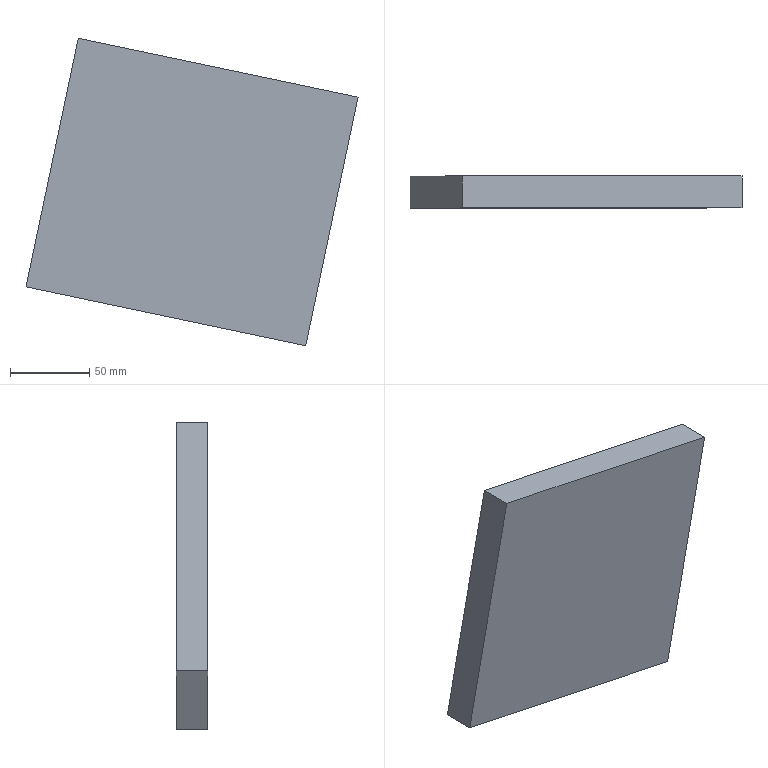Part | STEP file | 5_ESTAGIO_003-01 | 1 solid | 6 faces | box 209.056 x 20 x 193.596 mm | volume 576000 mm3 | plane 6
STEP:
#1=CARTESIAN_POINT('',(0.,0.,0.));
#2=DIRECTION('',(0.,0.,1.));
#3=DIRECTION('',(1.,0.,0.));
#4=AXIS2_PLACEMENT_3D('',#1,#2,#3);
#5=CARTESIAN_POINT('',(-2536.48,-709.15,1023.11));
#6=VERTEX_POINT('',#5);
#7=CARTESIAN_POINT('',(-2712.633,-709.15,1060.125));
#8=VERTEX_POINT('',#7);
#9=CARTESIAN_POINT('',(-2536.48,-709.15,1023.11));
#10=DIRECTION('',(-0.9786,0.,0.2056));
#11=VECTOR('',#10,1.);
#12=LINE('',#9,#11);
#13=CARTESIAN_POINT('',(-2536.48,-689.15,1023.11));
#14=DIRECTION('',(0.2056,0.,0.9786));
#15=DIRECTION('',(0.9786,0.,-0.2056));
#16=AXIS2_PLACEMENT_3D('',#13,#14,#15);
#17=PLANE('',#16);
#18=CARTESIAN_POINT('',(0.,-20.));
#19=DIRECTION('',(-1.,0.));
#20=VECTOR('',#19,1.);
#21=LINE('',#18,#20);
#22=(GEOMETRIC_REPRESENTATION_CONTEXT(2)PARAMETRIC_REPRESENTATION_CONTEXT()REPRESENTATION_CONTEXT('',''));
#23=DEFINITIONAL_REPRESENTATION('',(#21),#22);
#24=PCURVE('',#17,#23);
#25=CARTESIAN_POINT('',(0.,-709.15,0.));
#26=DIRECTION('',(0.,1.,0.));
#27=DIRECTION('',(0.,0.,1.));
#28=AXIS2_PLACEMENT_3D('',#25,#26,#27);
#29=PLANE('',#28);
#30=CARTESIAN_POINT('',(1023.11,-2536.48));
#31=DIRECTION('',(0.2056,-0.9786));
#32=VECTOR('',#31,1.);
#33=LINE('',#30,#32);
#34=(GEOMETRIC_REPRESENTATION_CONTEXT(2)PARAMETRIC_REPRESENTATION_CONTEXT()REPRESENTATION_CONTEXT('',''));
#35=DEFINITIONAL_REPRESENTATION('',(#33),#34);
#36=PCURVE('',#29,#35);
#37=SURFACE_CURVE('',#12,(#24,#36),.PCURVE_S1.);
#38=EDGE_CURVE('',#6,#8,#37,.T.);
#39=ORIENTED_EDGE('',*,*,#38,.F.);
#40=CARTESIAN_POINT('',(-2536.48,-689.15,1023.11));
#41=VERTEX_POINT('',#40);
#42=CARTESIAN_POINT('',(-2536.48,-689.15,1023.11));
#43=DIRECTION('',(0.,-1.,0.));
#44=VECTOR('',#43,1.);
#45=LINE('',#42,#44);
#46=CARTESIAN_POINT('',(0.,0.));
#47=DIRECTION('',(0.,-1.));
#48=VECTOR('',#47,1.);
#49=LINE('',#46,#48);
#50=(GEOMETRIC_REPRESENTATION_CONTEXT(2)PARAMETRIC_REPRESENTATION_CONTEXT()REPRESENTATION_CONTEXT('',''));
#51=DEFINITIONAL_REPRESENTATION('',(#49),#50);
#52=PCURVE('',#17,#51);
#53=CARTESIAN_POINT('',(-2569.383,-689.15,866.529));
#54=DIRECTION('',(0.9786,0.,-0.2056));
#55=DIRECTION('',(-0.2056,0.,-0.9786));
#56=AXIS2_PLACEMENT_3D('',#53,#54,#55);
#57=PLANE('',#56);
#58=CARTESIAN_POINT('',(-160.,0.));
#59=DIRECTION('',(0.,-1.));
#60=VECTOR('',#59,1.);
#61=LINE('',#58,#60);
#62=(GEOMETRIC_REPRESENTATION_CONTEXT(2)PARAMETRIC_REPRESENTATION_CONTEXT()REPRESENTATION_CONTEXT('',''));
#63=DEFINITIONAL_REPRESENTATION('',(#61),#62);
#64=PCURVE('',#57,#63);
#65=SURFACE_CURVE('',#45,(#52,#64),.PCURVE_S1.);
#66=EDGE_CURVE('',#41,#6,#65,.T.);
#67=ORIENTED_EDGE('',*,*,#66,.F.);
#68=CARTESIAN_POINT('',(-2712.633,-689.15,1060.125));
#69=VERTEX_POINT('',#68);
#70=CARTESIAN_POINT('',(-2536.48,-689.15,1023.11));
#71=DIRECTION('',(-0.9786,0.,0.2056));
#72=VECTOR('',#71,1.);
#73=LINE('',#70,#72);
#74=CARTESIAN_POINT('',(0.,0.));
#75=DIRECTION('',(-1.,0.));
#76=VECTOR('',#75,1.);
#77=LINE('',#74,#76);
#78=(GEOMETRIC_REPRESENTATION_CONTEXT(2)PARAMETRIC_REPRESENTATION_CONTEXT()REPRESENTATION_CONTEXT('',''));
#79=DEFINITIONAL_REPRESENTATION('',(#77),#78);
#80=PCURVE('',#17,#79);
#81=CARTESIAN_POINT('',(0.,-689.15,0.));
#82=DIRECTION('',(0.,1.,0.));
#83=DIRECTION('',(0.,0.,1.));
#84=AXIS2_PLACEMENT_3D('',#81,#82,#83);
#85=PLANE('',#84);
#86=CARTESIAN_POINT('',(1023.11,-2536.48));
#87=DIRECTION('',(0.2056,-0.9786));
#88=VECTOR('',#87,1.);
#89=LINE('',#86,#88);
#90=(GEOMETRIC_REPRESENTATION_CONTEXT(2)PARAMETRIC_REPRESENTATION_CONTEXT()REPRESENTATION_CONTEXT('',''));
#91=DEFINITIONAL_REPRESENTATION('',(#89),#90);
#92=PCURVE('',#85,#91);
#93=SURFACE_CURVE('',#73,(#80,#92),.PCURVE_S1.);
#94=EDGE_CURVE('',#41,#69,#93,.T.);
#95=ORIENTED_EDGE('',*,*,#94,.T.);
#96=CARTESIAN_POINT('',(-2712.633,-689.15,1060.125));
#97=DIRECTION('',(0.,-1.,0.));
#98=VECTOR('',#97,1.);
#99=LINE('',#96,#98);
#100=CARTESIAN_POINT('',(-180.,0.));
#101=DIRECTION('',(0.,-1.));
#102=VECTOR('',#101,1.);
#103=LINE('',#100,#102);
#104=(GEOMETRIC_REPRESENTATION_CONTEXT(2)PARAMETRIC_REPRESENTATION_CONTEXT()REPRESENTATION_CONTEXT('',''));
#105=DEFINITIONAL_REPRESENTATION('',(#103),#104);
#106=PCURVE('',#17,#105);
#107=CARTESIAN_POINT('',(-2712.633,-689.15,1060.125));
#108=DIRECTION('',(-0.9786,0.,0.2056));
#109=DIRECTION('',(0.2056,0.,0.9786));
#110=AXIS2_PLACEMENT_3D('',#107,#108,#109);
#111=PLANE('',#110);
#112=CARTESIAN_POINT('',(0.,0.));
#113=DIRECTION('',(0.,-1.));
#114=VECTOR('',#113,1.);
#115=LINE('',#112,#114);
#116=(GEOMETRIC_REPRESENTATION_CONTEXT(2)PARAMETRIC_REPRESENTATION_CONTEXT()REPRESENTATION_CONTEXT('',''));
#117=DEFINITIONAL_REPRESENTATION('',(#115),#116);
#118=PCURVE('',#111,#117);
#119=SURFACE_CURVE('',#99,(#106,#118),.PCURVE_S1.);
#120=EDGE_CURVE('',#69,#8,#119,.T.);
#121=ORIENTED_EDGE('',*,*,#120,.T.);
#122=EDGE_LOOP('',(#39,#67,#95,#121));
#123=FACE_BOUND('',#122,.T.);
#124=ADVANCED_FACE('',(#123),#17,.T.);
#125=CARTESIAN_POINT('',(-2569.383,-709.15,866.529));
#126=VERTEX_POINT('',#125);
#127=CARTESIAN_POINT('',(-2569.383,-709.15,866.529));
#128=DIRECTION('',(0.2056,0.,0.9786));
#129=VECTOR('',#128,1.);
#130=LINE('',#127,#129);
#131=CARTESIAN_POINT('',(0.,-20.));
#132=DIRECTION('',(-1.,0.));
#133=VECTOR('',#132,1.);
#134=LINE('',#131,#133);
#135=(GEOMETRIC_REPRESENTATION_CONTEXT(2)PARAMETRIC_REPRESENTATION_CONTEXT()REPRESENTATION_CONTEXT('',''));
#136=DEFINITIONAL_REPRESENTATION('',(#134),#135);
#137=PCURVE('',#57,#136);
#138=CARTESIAN_POINT('',(866.529,-2569.383));
#139=DIRECTION('',(0.9786,0.2056));
#140=VECTOR('',#139,1.);
#141=LINE('',#138,#140);
#142=(GEOMETRIC_REPRESENTATION_CONTEXT(2)PARAMETRIC_REPRESENTATION_CONTEXT()REPRESENTATION_CONTEXT('',''));
#143=DEFINITIONAL_REPRESENTATION('',(#141),#142);
#144=PCURVE('',#29,#143);
#145=SURFACE_CURVE('',#130,(#137,#144),.PCURVE_S1.);
#146=EDGE_CURVE('',#126,#6,#145,.T.);
#147=ORIENTED_EDGE('',*,*,#146,.F.);
#148=CARTESIAN_POINT('',(-2569.383,-689.15,866.529));
#149=VERTEX_POINT('',#148);
#150=CARTESIAN_POINT('',(-2569.383,-689.15,866.529));
#151=DIRECTION('',(0.,-1.,0.));
#152=VECTOR('',#151,1.);
#153=LINE('',#150,#152);
#154=CARTESIAN_POINT('',(0.,0.));
#155=DIRECTION('',(0.,-1.));
#156=VECTOR('',#155,1.);
#157=LINE('',#154,#156);
#158=(GEOMETRIC_REPRESENTATION_CONTEXT(2)PARAMETRIC_REPRESENTATION_CONTEXT()REPRESENTATION_CONTEXT('',''));
#159=DEFINITIONAL_REPRESENTATION('',(#157),#158);
#160=PCURVE('',#57,#159);
#161=CARTESIAN_POINT('',(-2745.535,-689.15,903.545));
#162=DIRECTION('',(-0.2056,0.,-0.9786));
#163=DIRECTION('',(-0.9786,0.,0.2056));
#164=AXIS2_PLACEMENT_3D('',#161,#162,#163);
#165=PLANE('',#164);
#166=CARTESIAN_POINT('',(-180.,0.));
#167=DIRECTION('',(0.,-1.));
#168=VECTOR('',#167,1.);
#169=LINE('',#166,#168);
#170=(GEOMETRIC_REPRESENTATION_CONTEXT(2)PARAMETRIC_REPRESENTATION_CONTEXT()REPRESENTATION_CONTEXT('',''));
#171=DEFINITIONAL_REPRESENTATION('',(#169),#170);
#172=PCURVE('',#165,#171);
#173=SURFACE_CURVE('',#153,(#160,#172),.PCURVE_S1.);
#174=EDGE_CURVE('',#149,#126,#173,.T.);
#175=ORIENTED_EDGE('',*,*,#174,.F.);
#176=CARTESIAN_POINT('',(-2569.383,-689.15,866.529));
#177=DIRECTION('',(0.2056,0.,0.9786));
#178=VECTOR('',#177,1.);
#179=LINE('',#176,#178);
#180=CARTESIAN_POINT('',(0.,0.));
#181=DIRECTION('',(-1.,0.));
#182=VECTOR('',#181,1.);
#183=LINE('',#180,#182);
#184=(GEOMETRIC_REPRESENTATION_CONTEXT(2)PARAMETRIC_REPRESENTATION_CONTEXT()REPRESENTATION_CONTEXT('',''));
#185=DEFINITIONAL_REPRESENTATION('',(#183),#184);
#186=PCURVE('',#57,#185);
#187=CARTESIAN_POINT('',(866.529,-2569.383));
#188=DIRECTION('',(0.9786,0.2056));
#189=VECTOR('',#188,1.);
#190=LINE('',#187,#189);
#191=(GEOMETRIC_REPRESENTATION_CONTEXT(2)PARAMETRIC_REPRESENTATION_CONTEXT()REPRESENTATION_CONTEXT('',''));
#192=DEFINITIONAL_REPRESENTATION('',(#190),#191);
#193=PCURVE('',#85,#192);
#194=SURFACE_CURVE('',#179,(#186,#193),.PCURVE_S1.);
#195=EDGE_CURVE('',#149,#41,#194,.T.);
#196=ORIENTED_EDGE('',*,*,#195,.T.);
#197=ORIENTED_EDGE('',*,*,#66,.T.);
#198=EDGE_LOOP('',(#147,#175,#196,#197));
#199=FACE_BOUND('',#198,.T.);
#200=ADVANCED_FACE('',(#199),#57,.T.);
#201=CARTESIAN_POINT('',(-2745.535,-709.15,903.545));
#202=VERTEX_POINT('',#201);
#203=CARTESIAN_POINT('',(-2745.535,-709.15,903.545));
#204=DIRECTION('',(0.9786,0.,-0.2056));
#205=VECTOR('',#204,1.);
#206=LINE('',#203,#205);
#207=CARTESIAN_POINT('',(0.,-20.));
#208=DIRECTION('',(-1.,0.));
#209=VECTOR('',#208,1.);
#210=LINE('',#207,#209);
#211=(GEOMETRIC_REPRESENTATION_CONTEXT(2)PARAMETRIC_REPRESENTATION_CONTEXT()REPRESENTATION_CONTEXT('',''));
#212=DEFINITIONAL_REPRESENTATION('',(#210),#211);
#213=PCURVE('',#165,#212);
#214=CARTESIAN_POINT('',(903.545,-2745.535));
#215=DIRECTION('',(-0.2056,0.9786));
#216=VECTOR('',#215,1.);
#217=LINE('',#214,#216);
#218=(GEOMETRIC_REPRESENTATION_CONTEXT(2)PARAMETRIC_REPRESENTATION_CONTEXT()REPRESENTATION_CONTEXT('',''));
#219=DEFINITIONAL_REPRESENTATION('',(#217),#218);
#220=PCURVE('',#29,#219);
#221=SURFACE_CURVE('',#206,(#213,#220),.PCURVE_S1.);
#222=EDGE_CURVE('',#202,#126,#221,.T.);
#223=ORIENTED_EDGE('',*,*,#222,.F.);
#224=CARTESIAN_POINT('',(-2745.535,-689.15,903.545));
#225=VERTEX_POINT('',#224);
#226=CARTESIAN_POINT('',(-2745.535,-689.15,903.545));
#227=DIRECTION('',(0.,-1.,0.));
#228=VECTOR('',#227,1.);
#229=LINE('',#226,#228);
#230=CARTESIAN_POINT('',(0.,0.));
#231=DIRECTION('',(0.,-1.));
#232=VECTOR('',#231,1.);
#233=LINE('',#230,#232);
#234=(GEOMETRIC_REPRESENTATION_CONTEXT(2)PARAMETRIC_REPRESENTATION_CONTEXT()REPRESENTATION_CONTEXT('',''));
#235=DEFINITIONAL_REPRESENTATION('',(#233),#234);
#236=PCURVE('',#165,#235);
#237=CARTESIAN_POINT('',(-160.,0.));
#238=DIRECTION('',(0.,-1.));
#239=VECTOR('',#238,1.);
#240=LINE('',#237,#239);
#241=(GEOMETRIC_REPRESENTATION_CONTEXT(2)PARAMETRIC_REPRESENTATION_CONTEXT()REPRESENTATION_CONTEXT('',''));
#242=DEFINITIONAL_REPRESENTATION('',(#240),#241);
#243=PCURVE('',#111,#242);
#244=SURFACE_CURVE('',#229,(#236,#243),.PCURVE_S1.);
#245=EDGE_CURVE('',#225,#202,#244,.T.);
#246=ORIENTED_EDGE('',*,*,#245,.F.);
#247=CARTESIAN_POINT('',(-2745.535,-689.15,903.545));
#248=DIRECTION('',(0.9786,0.,-0.2056));
#249=VECTOR('',#248,1.);
#250=LINE('',#247,#249);
#251=CARTESIAN_POINT('',(0.,0.));
#252=DIRECTION('',(-1.,0.));
#253=VECTOR('',#252,1.);
#254=LINE('',#251,#253);
#255=(GEOMETRIC_REPRESENTATION_CONTEXT(2)PARAMETRIC_REPRESENTATION_CONTEXT()REPRESENTATION_CONTEXT('',''));
#256=DEFINITIONAL_REPRESENTATION('',(#254),#255);
#257=PCURVE('',#165,#256);
#258=CARTESIAN_POINT('',(903.545,-2745.535));
#259=DIRECTION('',(-0.2056,0.9786));
#260=VECTOR('',#259,1.);
#261=LINE('',#258,#260);
#262=(GEOMETRIC_REPRESENTATION_CONTEXT(2)PARAMETRIC_REPRESENTATION_CONTEXT()REPRESENTATION_CONTEXT('',''));
#263=DEFINITIONAL_REPRESENTATION('',(#261),#262);
#264=PCURVE('',#85,#263);
#265=SURFACE_CURVE('',#250,(#257,#264),.PCURVE_S1.);
#266=EDGE_CURVE('',#225,#149,#265,.T.);
#267=ORIENTED_EDGE('',*,*,#266,.T.);
#268=ORIENTED_EDGE('',*,*,#174,.T.);
#269=EDGE_LOOP('',(#223,#246,#267,#268));
#270=FACE_BOUND('',#269,.T.);
#271=ADVANCED_FACE('',(#270),#165,.T.);
#272=CARTESIAN_POINT('',(-2712.633,-709.15,1060.125));
#273=DIRECTION('',(-0.2056,0.,-0.9786));
#274=VECTOR('',#273,1.);
#275=LINE('',#272,#274);
#276=CARTESIAN_POINT('',(-0.000000001,-20.));
#277=DIRECTION('',(-1.,0.));
#278=VECTOR('',#277,1.);
#279=LINE('',#276,#278);
#280=(GEOMETRIC_REPRESENTATION_CONTEXT(2)PARAMETRIC_REPRESENTATION_CONTEXT()REPRESENTATION_CONTEXT('',''));
#281=DEFINITIONAL_REPRESENTATION('',(#279),#280);
#282=PCURVE('',#111,#281);
#283=CARTESIAN_POINT('',(1060.125,-2712.633));
#284=DIRECTION('',(-0.9786,-0.2056));
#285=VECTOR('',#284,1.);
#286=LINE('',#283,#285);
#287=(GEOMETRIC_REPRESENTATION_CONTEXT(2)PARAMETRIC_REPRESENTATION_CONTEXT()REPRESENTATION_CONTEXT('',''));
#288=DEFINITIONAL_REPRESENTATION('',(#286),#287);
#289=PCURVE('',#29,#288);
#290=SURFACE_CURVE('',#275,(#282,#289),.PCURVE_S1.);
#291=EDGE_CURVE('',#8,#202,#290,.T.);
#292=ORIENTED_EDGE('',*,*,#291,.F.);
#293=ORIENTED_EDGE('',*,*,#120,.F.);
#294=CARTESIAN_POINT('',(-2712.633,-689.15,1060.125));
#295=DIRECTION('',(-0.2056,0.,-0.9786));
#296=VECTOR('',#295,1.);
#297=LINE('',#294,#296);
#298=CARTESIAN_POINT('',(-0.000000001,0.));
#299=DIRECTION('',(-1.,0.));
#300=VECTOR('',#299,1.);
#301=LINE('',#298,#300);
#302=(GEOMETRIC_REPRESENTATION_CONTEXT(2)PARAMETRIC_REPRESENTATION_CONTEXT()REPRESENTATION_CONTEXT('',''));
#303=DEFINITIONAL_REPRESENTATION('',(#301),#302);
#304=PCURVE('',#111,#303);
#305=CARTESIAN_POINT('',(1060.125,-2712.633));
#306=DIRECTION('',(-0.9786,-0.2056));
#307=VECTOR('',#306,1.);
#308=LINE('',#305,#307);
#309=(GEOMETRIC_REPRESENTATION_CONTEXT(2)PARAMETRIC_REPRESENTATION_CONTEXT()REPRESENTATION_CONTEXT('',''));
#310=DEFINITIONAL_REPRESENTATION('',(#308),#309);
#311=PCURVE('',#85,#310);
#312=SURFACE_CURVE('',#297,(#304,#311),.PCURVE_S1.);
#313=EDGE_CURVE('',#69,#225,#312,.T.);
#314=ORIENTED_EDGE('',*,*,#313,.T.);
#315=ORIENTED_EDGE('',*,*,#245,.T.);
#316=EDGE_LOOP('',(#292,#293,#314,#315));
#317=FACE_BOUND('',#316,.T.);
#318=ADVANCED_FACE('',(#317),#111,.T.);
#319=ORIENTED_EDGE('',*,*,#94,.F.);
#320=ORIENTED_EDGE('',*,*,#195,.F.);
#321=ORIENTED_EDGE('',*,*,#266,.F.);
#322=ORIENTED_EDGE('',*,*,#313,.F.);
#323=EDGE_LOOP('',(#319,#320,#321,#322));
#324=FACE_BOUND('',#323,.T.);
#325=ADVANCED_FACE('',(#324),#85,.T.);
#326=ORIENTED_EDGE('',*,*,#291,.T.);
#327=ORIENTED_EDGE('',*,*,#222,.T.);
#328=ORIENTED_EDGE('',*,*,#146,.T.);
#329=ORIENTED_EDGE('',*,*,#38,.T.);
#330=EDGE_LOOP('',(#326,#327,#328,#329));
#331=FACE_BOUND('',#330,.T.);
#332=ADVANCED_FACE('',(#331),#29,.F.);
#333=CLOSED_SHELL('',(#124,#200,#271,#318,#325,#332));
#334=MANIFOLD_SOLID_BREP('',#333);
#335=(LENGTH_UNIT()NAMED_UNIT(*)SI_UNIT(.MILLI.,.METRE.));
#336=UNCERTAINTY_MEASURE_WITH_UNIT(LENGTH_MEASURE(0.0000001),#335,'','');
#337=(NAMED_UNIT(*)PLANE_ANGLE_UNIT()SI_UNIT($,.RADIAN.));
#338=(NAMED_UNIT(*)SI_UNIT($,.STERADIAN.)SOLID_ANGLE_UNIT());
#339=(GEOMETRIC_REPRESENTATION_CONTEXT(3)GLOBAL_UNCERTAINTY_ASSIGNED_CONTEXT((#336))GLOBAL_UNIT_ASSIGNED_CONTEXT((#335,#337,#338))REPRESENTATION_CONTEXT('',''));
#340=ADVANCED_BREP_SHAPE_REPRESENTATION('',(#4,#334),#339);